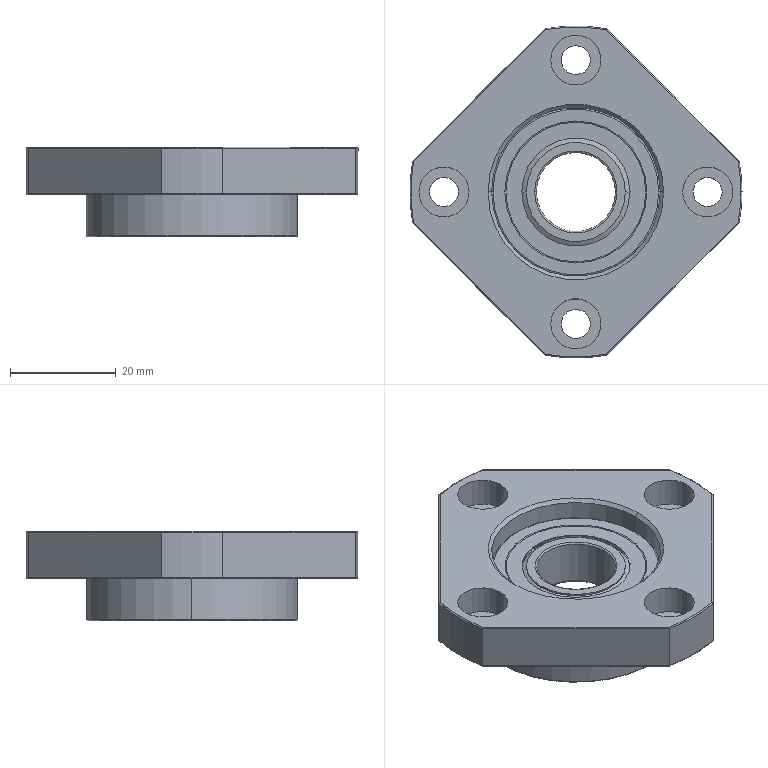Part | SolidWorks | features BaseBody 14 | 14 solids | 258 faces | box 63 x 63 x 17 mm | volume 21756 mm3 | cylinder 91 | sphere 84 | plane 41 | torus 34 | cone 8 | commonest cylinder face diameters 22.95 x21 24.05 x21 0.44 x8 5.5 x8 9.5 x8 63 x5